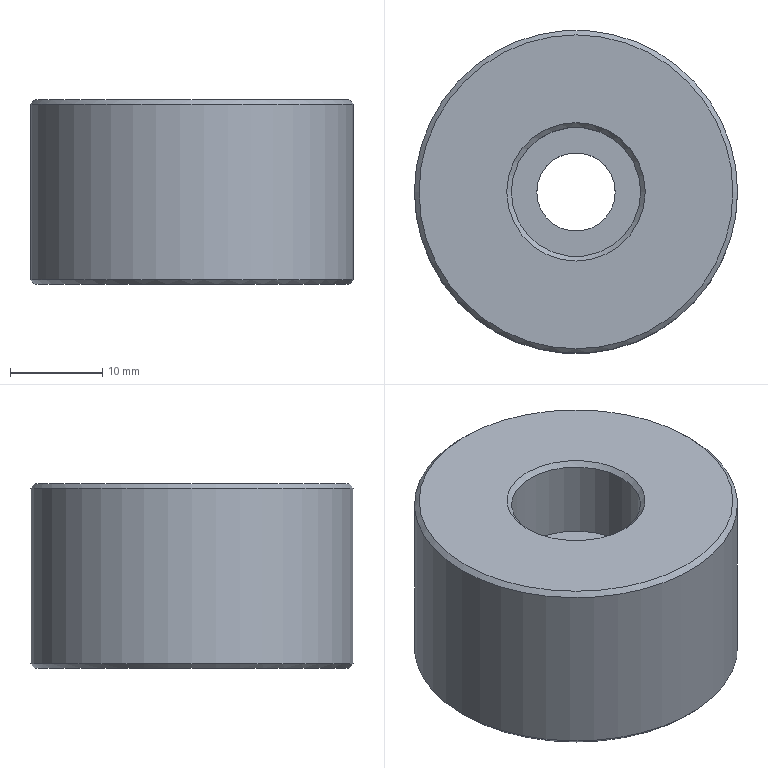Part | STEP file | solid 89 | 1 solid | 9 faces | box 35 x 35 x 20 mm | volume 17200 mm3 | plane 3 | cylinder 3 | cone 3 | commonest cylinder face diameters 8.5 x1 14 x1 35 x1